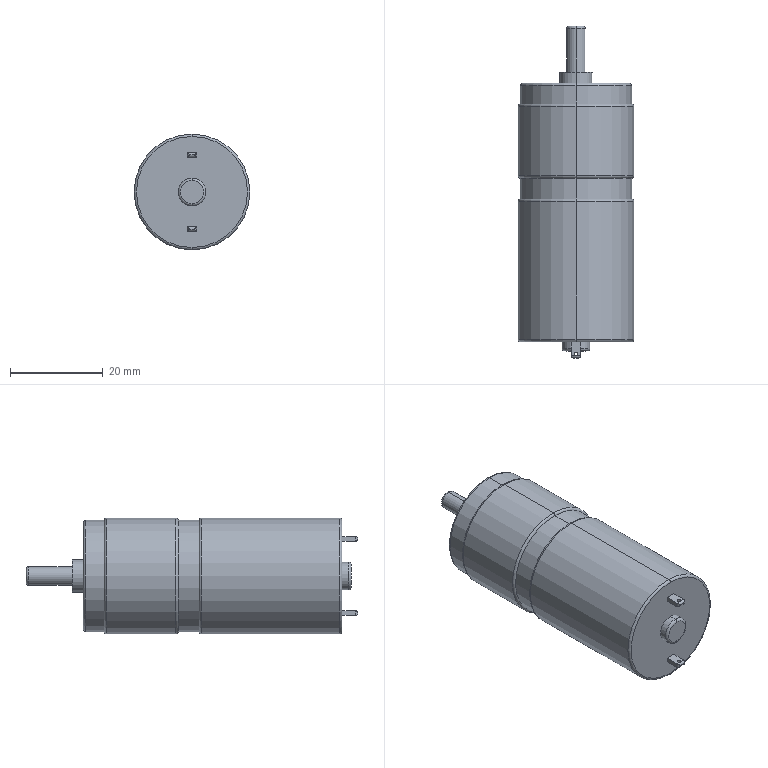Part | STEP file | 370 straight motor | 1 solid | 59 faces | box 25 x 71.68 x 25 mm | volume 27082 mm3 | cylinder 30 | plane 15 | torus 14 | commonest cylinder face diameters 1 x8 0.834 x4 3 x4 24 x4 25 x4 4 x2